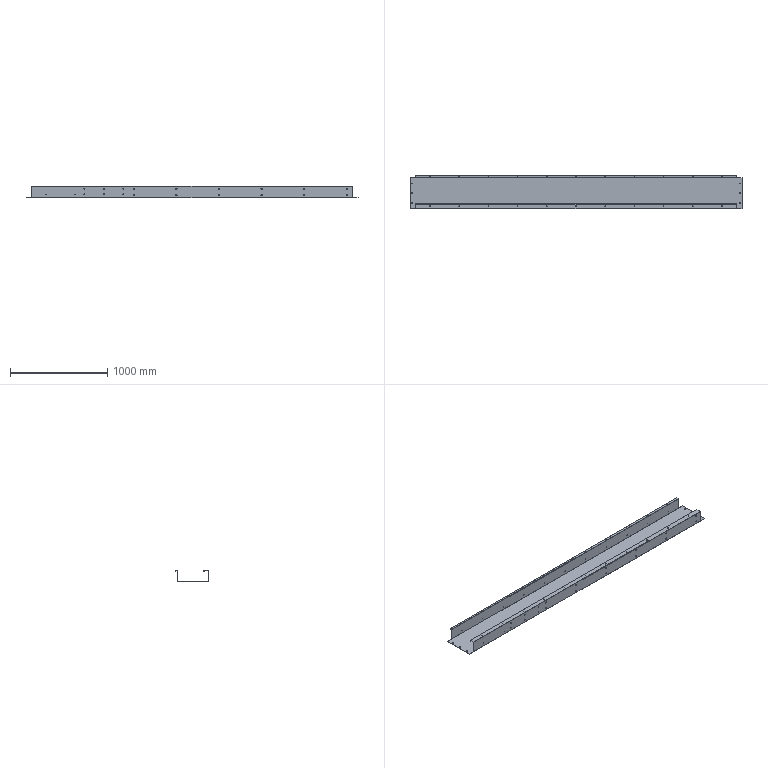Part | STEP file | SX-001-01 | 1 solid | 237 faces | box 3411 x 343 x 122 mm | volume 4398999 mm3 | cylinder 132 | plane 105 | commonest cylinder face diameters 5.4 x48 10 x24 8 x22 7 x12 10.5 x12 0.4 x6